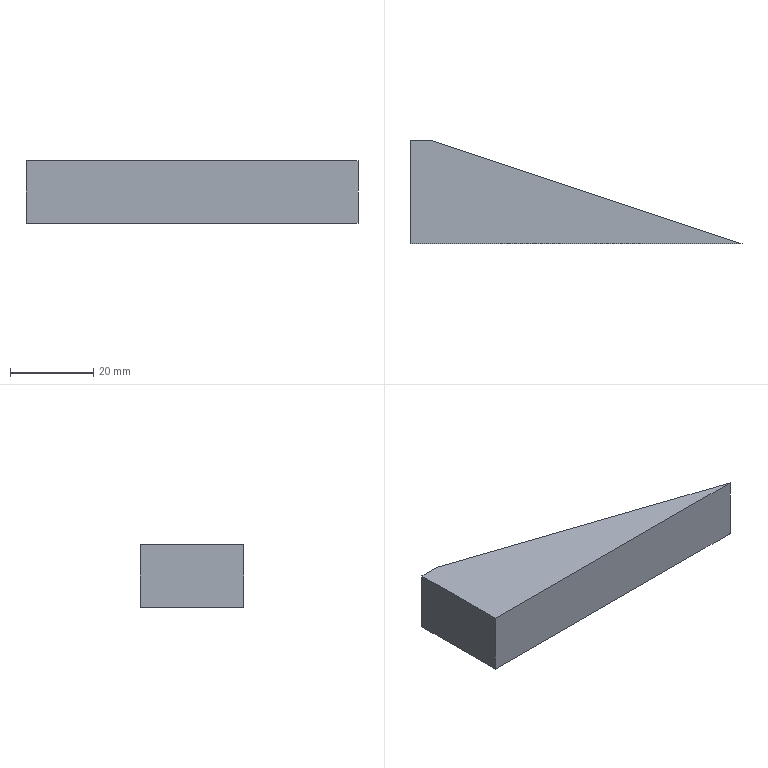Part | STEP file | 001-011-Blanking flip straightening block | 1 solid | 6 faces | box 80 x 25 x 15 mm | volume 15938 mm3 | plane 6
STEP:
#1=CARTESIAN_POINT('',(0.,0.,0.));
#2=DIRECTION('',(0.,0.,1.));
#3=DIRECTION('',(1.,0.,0.));
#4=AXIS2_PLACEMENT_3D('',#1,#2,#3);
#5=CARTESIAN_POINT('',(-35.,12.5,15.));
#6=VERTEX_POINT('',#5);
#7=CARTESIAN_POINT('',(-40.,12.5,15.));
#8=VERTEX_POINT('',#7);
#9=CARTESIAN_POINT('',(-40.,12.5,15.));
#10=DIRECTION('',(-1.,0.,0.));
#11=VECTOR('',#10,1.);
#12=LINE('',#9,#11);
#13=CARTESIAN_POINT('',(-40.,12.5,15.));
#14=DIRECTION('',(0.,-1.,0.));
#15=DIRECTION('',(1.,0.,0.));
#16=AXIS2_PLACEMENT_3D('',#13,#14,#15);
#17=PLANE('',#16);
#18=CARTESIAN_POINT('',(0.,0.));
#19=DIRECTION('',(-1.,0.));
#20=VECTOR('',#19,1.);
#21=LINE('',#18,#20);
#22=(GEOMETRIC_REPRESENTATION_CONTEXT(2)PARAMETRIC_REPRESENTATION_CONTEXT()REPRESENTATION_CONTEXT('',''));
#23=DEFINITIONAL_REPRESENTATION('',(#21),#22);
#24=PCURVE('',#17,#23);
#25=CARTESIAN_POINT('',(0.,0.,15.));
#26=DIRECTION('',(0.,0.,-1.));
#27=DIRECTION('',(-1.,0.,0.));
#28=AXIS2_PLACEMENT_3D('',#25,#26,#27);
#29=PLANE('',#28);
#30=CARTESIAN_POINT('',(40.,12.5));
#31=DIRECTION('',(1.,0.));
#32=VECTOR('',#31,1.);
#33=LINE('',#30,#32);
#34=(GEOMETRIC_REPRESENTATION_CONTEXT(2)PARAMETRIC_REPRESENTATION_CONTEXT()REPRESENTATION_CONTEXT('',''));
#35=DEFINITIONAL_REPRESENTATION('',(#33),#34);
#36=PCURVE('',#29,#35);
#37=SURFACE_CURVE('',#12,(#24,#36),.PCURVE_S1.);
#38=EDGE_CURVE('',#6,#8,#37,.T.);
#39=ORIENTED_EDGE('',*,*,#38,.F.);
#40=CARTESIAN_POINT('',(-35.,12.5,0.));
#41=VERTEX_POINT('',#40);
#42=CARTESIAN_POINT('',(-35.,12.5,0.));
#43=DIRECTION('',(0.,0.,1.));
#44=VECTOR('',#43,1.);
#45=LINE('',#42,#44);
#46=CARTESIAN_POINT('',(5.,-15.));
#47=DIRECTION('',(0.,1.));
#48=VECTOR('',#47,1.);
#49=LINE('',#46,#48);
#50=(GEOMETRIC_REPRESENTATION_CONTEXT(2)PARAMETRIC_REPRESENTATION_CONTEXT()REPRESENTATION_CONTEXT('',''));
#51=DEFINITIONAL_REPRESENTATION('',(#49),#50);
#52=PCURVE('',#17,#51);
#53=CARTESIAN_POINT('',(40.,-12.5,0.));
#54=DIRECTION('',(-0.3162,-0.9487,0.));
#55=DIRECTION('',(0.9487,-0.3162,0.));
#56=AXIS2_PLACEMENT_3D('',#53,#54,#55);
#57=PLANE('',#56);
#58=CARTESIAN_POINT('',(-79.057,0.));
#59=DIRECTION('',(0.,1.));
#60=VECTOR('',#59,1.);
#61=LINE('',#58,#60);
#62=(GEOMETRIC_REPRESENTATION_CONTEXT(2)PARAMETRIC_REPRESENTATION_CONTEXT()REPRESENTATION_CONTEXT('',''));
#63=DEFINITIONAL_REPRESENTATION('',(#61),#62);
#64=PCURVE('',#57,#63);
#65=SURFACE_CURVE('',#45,(#52,#64),.PCURVE_S1.);
#66=EDGE_CURVE('',#41,#6,#65,.T.);
#67=ORIENTED_EDGE('',*,*,#66,.F.);
#68=CARTESIAN_POINT('',(-40.,12.5,0.));
#69=VERTEX_POINT('',#68);
#70=CARTESIAN_POINT('',(-40.,12.5,0.));
#71=DIRECTION('',(-1.,0.,0.));
#72=VECTOR('',#71,1.);
#73=LINE('',#70,#72);
#74=CARTESIAN_POINT('',(0.,-15.));
#75=DIRECTION('',(-1.,0.));
#76=VECTOR('',#75,1.);
#77=LINE('',#74,#76);
#78=(GEOMETRIC_REPRESENTATION_CONTEXT(2)PARAMETRIC_REPRESENTATION_CONTEXT()REPRESENTATION_CONTEXT('',''));
#79=DEFINITIONAL_REPRESENTATION('',(#77),#78);
#80=PCURVE('',#17,#79);
#81=CARTESIAN_POINT('',(0.,0.,0.));
#82=DIRECTION('',(0.,0.,-1.));
#83=DIRECTION('',(-1.,0.,0.));
#84=AXIS2_PLACEMENT_3D('',#81,#82,#83);
#85=PLANE('',#84);
#86=CARTESIAN_POINT('',(40.,12.5));
#87=DIRECTION('',(1.,0.));
#88=VECTOR('',#87,1.);
#89=LINE('',#86,#88);
#90=(GEOMETRIC_REPRESENTATION_CONTEXT(2)PARAMETRIC_REPRESENTATION_CONTEXT()REPRESENTATION_CONTEXT('',''));
#91=DEFINITIONAL_REPRESENTATION('',(#89),#90);
#92=PCURVE('',#85,#91);
#93=SURFACE_CURVE('',#73,(#80,#92),.PCURVE_S1.);
#94=EDGE_CURVE('',#41,#69,#93,.T.);
#95=ORIENTED_EDGE('',*,*,#94,.T.);
#96=CARTESIAN_POINT('',(-40.,12.5,15.));
#97=DIRECTION('',(0.,0.,-1.));
#98=VECTOR('',#97,1.);
#99=LINE('',#96,#98);
#100=CARTESIAN_POINT('',(0.,0.));
#101=DIRECTION('',(0.,-1.));
#102=VECTOR('',#101,1.);
#103=LINE('',#100,#102);
#104=(GEOMETRIC_REPRESENTATION_CONTEXT(2)PARAMETRIC_REPRESENTATION_CONTEXT()REPRESENTATION_CONTEXT('',''));
#105=DEFINITIONAL_REPRESENTATION('',(#103),#104);
#106=PCURVE('',#17,#105);
#107=CARTESIAN_POINT('',(-40.,-12.5,15.));
#108=DIRECTION('',(1.,0.,0.));
#109=DIRECTION('',(0.,0.,-1.));
#110=AXIS2_PLACEMENT_3D('',#107,#108,#109);
#111=PLANE('',#110);
#112=CARTESIAN_POINT('',(0.,25.));
#113=DIRECTION('',(1.,0.));
#114=VECTOR('',#113,1.);
#115=LINE('',#112,#114);
#116=(GEOMETRIC_REPRESENTATION_CONTEXT(2)PARAMETRIC_REPRESENTATION_CONTEXT()REPRESENTATION_CONTEXT('',''));
#117=DEFINITIONAL_REPRESENTATION('',(#115),#116);
#118=PCURVE('',#111,#117);
#119=SURFACE_CURVE('',#99,(#106,#118),.PCURVE_S1.);
#120=EDGE_CURVE('',#8,#69,#119,.T.);
#121=ORIENTED_EDGE('',*,*,#120,.F.);
#122=EDGE_LOOP('',(#39,#67,#95,#121));
#123=FACE_BOUND('',#122,.T.);
#124=ADVANCED_FACE('',(#123),#17,.F.);
#125=CARTESIAN_POINT('',(-40.,-12.5,0.));
#126=VERTEX_POINT('',#125);
#127=CARTESIAN_POINT('',(-40.,-12.5,0.));
#128=DIRECTION('',(0.,-1.,0.));
#129=VECTOR('',#128,1.);
#130=LINE('',#127,#129);
#131=CARTESIAN_POINT('',(15.,0.));
#132=DIRECTION('',(0.,-1.));
#133=VECTOR('',#132,1.);
#134=LINE('',#131,#133);
#135=(GEOMETRIC_REPRESENTATION_CONTEXT(2)PARAMETRIC_REPRESENTATION_CONTEXT()REPRESENTATION_CONTEXT('',''));
#136=DEFINITIONAL_REPRESENTATION('',(#134),#135);
#137=PCURVE('',#111,#136);
#138=CARTESIAN_POINT('',(40.,-12.5));
#139=DIRECTION('',(0.,-1.));
#140=VECTOR('',#139,1.);
#141=LINE('',#138,#140);
#142=(GEOMETRIC_REPRESENTATION_CONTEXT(2)PARAMETRIC_REPRESENTATION_CONTEXT()REPRESENTATION_CONTEXT('',''));
#143=DEFINITIONAL_REPRESENTATION('',(#141),#142);
#144=PCURVE('',#85,#143);
#145=SURFACE_CURVE('',#130,(#137,#144),.PCURVE_S1.);
#146=EDGE_CURVE('',#69,#126,#145,.T.);
#147=ORIENTED_EDGE('',*,*,#146,.T.);
#148=CARTESIAN_POINT('',(-40.,-12.5,15.));
#149=VERTEX_POINT('',#148);
#150=CARTESIAN_POINT('',(-40.,-12.5,15.));
#151=DIRECTION('',(0.,0.,-1.));
#152=VECTOR('',#151,1.);
#153=LINE('',#150,#152);
#154=CARTESIAN_POINT('',(0.,0.));
#155=DIRECTION('',(1.,0.));
#156=VECTOR('',#155,1.);
#157=LINE('',#154,#156);
#158=(GEOMETRIC_REPRESENTATION_CONTEXT(2)PARAMETRIC_REPRESENTATION_CONTEXT()REPRESENTATION_CONTEXT('',''));
#159=DEFINITIONAL_REPRESENTATION('',(#157),#158);
#160=PCURVE('',#111,#159);
#161=CARTESIAN_POINT('',(-40.,-12.5,15.));
#162=DIRECTION('',(0.,1.,0.));
#163=DIRECTION('',(-1.,0.,0.));
#164=AXIS2_PLACEMENT_3D('',#161,#162,#163);
#165=PLANE('',#164);
#166=CARTESIAN_POINT('',(0.,0.));
#167=DIRECTION('',(0.,-1.));
#168=VECTOR('',#167,1.);
#169=LINE('',#166,#168);
#170=(GEOMETRIC_REPRESENTATION_CONTEXT(2)PARAMETRIC_REPRESENTATION_CONTEXT()REPRESENTATION_CONTEXT('',''));
#171=DEFINITIONAL_REPRESENTATION('',(#169),#170);
#172=PCURVE('',#165,#171);
#173=SURFACE_CURVE('',#153,(#160,#172),.PCURVE_S1.);
#174=EDGE_CURVE('',#149,#126,#173,.T.);
#175=ORIENTED_EDGE('',*,*,#174,.F.);
#176=CARTESIAN_POINT('',(-40.,-12.5,15.));
#177=DIRECTION('',(0.,-1.,0.));
#178=VECTOR('',#177,1.);
#179=LINE('',#176,#178);
#180=CARTESIAN_POINT('',(0.,0.));
#181=DIRECTION('',(0.,-1.));
#182=VECTOR('',#181,1.);
#183=LINE('',#180,#182);
#184=(GEOMETRIC_REPRESENTATION_CONTEXT(2)PARAMETRIC_REPRESENTATION_CONTEXT()REPRESENTATION_CONTEXT('',''));
#185=DEFINITIONAL_REPRESENTATION('',(#183),#184);
#186=PCURVE('',#111,#185);
#187=CARTESIAN_POINT('',(40.,-12.5));
#188=DIRECTION('',(0.,-1.));
#189=VECTOR('',#188,1.);
#190=LINE('',#187,#189);
#191=(GEOMETRIC_REPRESENTATION_CONTEXT(2)PARAMETRIC_REPRESENTATION_CONTEXT()REPRESENTATION_CONTEXT('',''));
#192=DEFINITIONAL_REPRESENTATION('',(#190),#191);
#193=PCURVE('',#29,#192);
#194=SURFACE_CURVE('',#179,(#186,#193),.PCURVE_S1.);
#195=EDGE_CURVE('',#8,#149,#194,.T.);
#196=ORIENTED_EDGE('',*,*,#195,.F.);
#197=ORIENTED_EDGE('',*,*,#120,.T.);
#198=EDGE_LOOP('',(#147,#175,#196,#197));
#199=FACE_BOUND('',#198,.T.);
#200=ADVANCED_FACE('',(#199),#111,.F.);
#201=CARTESIAN_POINT('',(40.,-12.5,0.));
#202=VERTEX_POINT('',#201);
#203=CARTESIAN_POINT('',(-40.,-12.5,0.));
#204=DIRECTION('',(1.,0.,0.));
#205=VECTOR('',#204,1.);
#206=LINE('',#203,#205);
#207=CARTESIAN_POINT('',(0.,-15.));
#208=DIRECTION('',(-1.,0.));
#209=VECTOR('',#208,1.);
#210=LINE('',#207,#209);
#211=(GEOMETRIC_REPRESENTATION_CONTEXT(2)PARAMETRIC_REPRESENTATION_CONTEXT()REPRESENTATION_CONTEXT('',''));
#212=DEFINITIONAL_REPRESENTATION('',(#210),#211);
#213=PCURVE('',#165,#212);
#214=CARTESIAN_POINT('',(40.,-12.5));
#215=DIRECTION('',(-1.,0.));
#216=VECTOR('',#215,1.);
#217=LINE('',#214,#216);
#218=(GEOMETRIC_REPRESENTATION_CONTEXT(2)PARAMETRIC_REPRESENTATION_CONTEXT()REPRESENTATION_CONTEXT('',''));
#219=DEFINITIONAL_REPRESENTATION('',(#217),#218);
#220=PCURVE('',#85,#219);
#221=SURFACE_CURVE('',#206,(#213,#220),.PCURVE_S1.);
#222=EDGE_CURVE('',#126,#202,#221,.T.);
#223=ORIENTED_EDGE('',*,*,#222,.T.);
#224=CARTESIAN_POINT('',(40.,-12.5,15.));
#225=VERTEX_POINT('',#224);
#226=CARTESIAN_POINT('',(40.,-12.5,15.));
#227=DIRECTION('',(0.,0.,-1.));
#228=VECTOR('',#227,1.);
#229=LINE('',#226,#228);
#230=CARTESIAN_POINT('',(-80.,0.));
#231=DIRECTION('',(0.,-1.));
#232=VECTOR('',#231,1.);
#233=LINE('',#230,#232);
#234=(GEOMETRIC_REPRESENTATION_CONTEXT(2)PARAMETRIC_REPRESENTATION_CONTEXT()REPRESENTATION_CONTEXT('',''));
#235=DEFINITIONAL_REPRESENTATION('',(#233),#234);
#236=PCURVE('',#165,#235);
#237=CARTESIAN_POINT('',(0.,15.));
#238=DIRECTION('',(0.,-1.));
#239=VECTOR('',#238,1.);
#240=LINE('',#237,#239);
#241=(GEOMETRIC_REPRESENTATION_CONTEXT(2)PARAMETRIC_REPRESENTATION_CONTEXT()REPRESENTATION_CONTEXT('',''));
#242=DEFINITIONAL_REPRESENTATION('',(#240),#241);
#243=PCURVE('',#57,#242);
#244=SURFACE_CURVE('',#229,(#236,#243),.PCURVE_S1.);
#245=EDGE_CURVE('',#225,#202,#244,.T.);
#246=ORIENTED_EDGE('',*,*,#245,.F.);
#247=CARTESIAN_POINT('',(-40.,-12.5,15.));
#248=DIRECTION('',(1.,0.,0.));
#249=VECTOR('',#248,1.);
#250=LINE('',#247,#249);
#251=CARTESIAN_POINT('',(0.,0.));
#252=DIRECTION('',(-1.,0.));
#253=VECTOR('',#252,1.);
#254=LINE('',#251,#253);
#255=(GEOMETRIC_REPRESENTATION_CONTEXT(2)PARAMETRIC_REPRESENTATION_CONTEXT()REPRESENTATION_CONTEXT('',''));
#256=DEFINITIONAL_REPRESENTATION('',(#254),#255);
#257=PCURVE('',#165,#256);
#258=CARTESIAN_POINT('',(40.,-12.5));
#259=DIRECTION('',(-1.,0.));
#260=VECTOR('',#259,1.);
#261=LINE('',#258,#260);
#262=(GEOMETRIC_REPRESENTATION_CONTEXT(2)PARAMETRIC_REPRESENTATION_CONTEXT()REPRESENTATION_CONTEXT('',''));
#263=DEFINITIONAL_REPRESENTATION('',(#261),#262);
#264=PCURVE('',#29,#263);
#265=SURFACE_CURVE('',#250,(#257,#264),.PCURVE_S1.);
#266=EDGE_CURVE('',#149,#225,#265,.T.);
#267=ORIENTED_EDGE('',*,*,#266,.F.);
#268=ORIENTED_EDGE('',*,*,#174,.T.);
#269=EDGE_LOOP('',(#223,#246,#267,#268));
#270=FACE_BOUND('',#269,.T.);
#271=ADVANCED_FACE('',(#270),#165,.F.);
#272=ORIENTED_EDGE('',*,*,#266,.T.);
#273=CARTESIAN_POINT('',(0.25,0.75,15.));
#274=DIRECTION('',(-0.9487,0.3162,0.));
#275=VECTOR('',#274,1.);
#276=LINE('',#273,#275);
#277=CARTESIAN_POINT('',(-0.25,0.75));
#278=DIRECTION('',(0.9487,0.3162));
#279=VECTOR('',#278,1.);
#280=LINE('',#277,#279);
#281=(GEOMETRIC_REPRESENTATION_CONTEXT(2)PARAMETRIC_REPRESENTATION_CONTEXT()REPRESENTATION_CONTEXT('',''));
#282=DEFINITIONAL_REPRESENTATION('',(#280),#281);
#283=PCURVE('',#29,#282);
#284=CARTESIAN_POINT('',(-41.9,15.));
#285=DIRECTION('',(-1.,0.));
#286=VECTOR('',#285,1.);
#287=LINE('',#284,#286);
#288=(GEOMETRIC_REPRESENTATION_CONTEXT(2)PARAMETRIC_REPRESENTATION_CONTEXT()REPRESENTATION_CONTEXT('',''));
#289=DEFINITIONAL_REPRESENTATION('',(#287),#288);
#290=PCURVE('',#57,#289);
#291=SURFACE_CURVE('',#276,(#283,#290),.PCURVE_S1.);
#292=EDGE_CURVE('',#225,#6,#291,.T.);
#293=ORIENTED_EDGE('',*,*,#292,.T.);
#294=ORIENTED_EDGE('',*,*,#38,.T.);
#295=ORIENTED_EDGE('',*,*,#195,.T.);
#296=EDGE_LOOP('',(#272,#293,#294,#295));
#297=FACE_BOUND('',#296,.T.);
#298=ADVANCED_FACE('',(#297),#29,.F.);
#299=CARTESIAN_POINT('',(40.,-12.5,0.));
#300=DIRECTION('',(0.9487,-0.3162,0.));
#301=VECTOR('',#300,1.);
#302=LINE('',#299,#301);
#303=CARTESIAN_POINT('',(-40.,-12.5));
#304=DIRECTION('',(-0.9487,-0.3162));
#305=VECTOR('',#304,1.);
#306=LINE('',#303,#305);
#307=(GEOMETRIC_REPRESENTATION_CONTEXT(2)PARAMETRIC_REPRESENTATION_CONTEXT()REPRESENTATION_CONTEXT('',''));
#308=DEFINITIONAL_REPRESENTATION('',(#306),#307);
#309=PCURVE('',#85,#308);
#310=CARTESIAN_POINT('',(0.,0.));
#311=DIRECTION('',(1.,0.));
#312=VECTOR('',#311,1.);
#313=LINE('',#310,#312);
#314=(GEOMETRIC_REPRESENTATION_CONTEXT(2)PARAMETRIC_REPRESENTATION_CONTEXT()REPRESENTATION_CONTEXT('',''));
#315=DEFINITIONAL_REPRESENTATION('',(#313),#314);
#316=PCURVE('',#57,#315);
#317=SURFACE_CURVE('',#302,(#309,#316),.PCURVE_S1.);
#318=EDGE_CURVE('',#41,#202,#317,.T.);
#319=ORIENTED_EDGE('',*,*,#318,.T.);
#320=ORIENTED_EDGE('',*,*,#222,.F.);
#321=ORIENTED_EDGE('',*,*,#146,.F.);
#322=ORIENTED_EDGE('',*,*,#94,.F.);
#323=EDGE_LOOP('',(#319,#320,#321,#322));
#324=FACE_BOUND('',#323,.T.);
#325=ADVANCED_FACE('',(#324),#85,.T.);
#326=ORIENTED_EDGE('',*,*,#245,.T.);
#327=ORIENTED_EDGE('',*,*,#318,.F.);
#328=ORIENTED_EDGE('',*,*,#66,.T.);
#329=ORIENTED_EDGE('',*,*,#292,.F.);
#330=EDGE_LOOP('',(#326,#327,#328,#329));
#331=FACE_BOUND('',#330,.T.);
#332=ADVANCED_FACE('',(#331),#57,.F.);
#333=CLOSED_SHELL('',(#124,#200,#271,#298,#325,#332));
#334=MANIFOLD_SOLID_BREP('',#333);
#335=(LENGTH_UNIT()NAMED_UNIT(*)SI_UNIT(.MILLI.,.METRE.));
#336=UNCERTAINTY_MEASURE_WITH_UNIT(LENGTH_MEASURE(0.0000005),#335,'','');
#337=(NAMED_UNIT(*)PLANE_ANGLE_UNIT()SI_UNIT($,.RADIAN.));
#338=(NAMED_UNIT(*)SI_UNIT($,.STERADIAN.)SOLID_ANGLE_UNIT());
#339=(GEOMETRIC_REPRESENTATION_CONTEXT(3)GLOBAL_UNCERTAINTY_ASSIGNED_CONTEXT((#336))GLOBAL_UNIT_ASSIGNED_CONTEXT((#335,#337,#338))REPRESENTATION_CONTEXT('',''));
#340=ADVANCED_BREP_SHAPE_REPRESENTATION('',(#4,#334),#339);